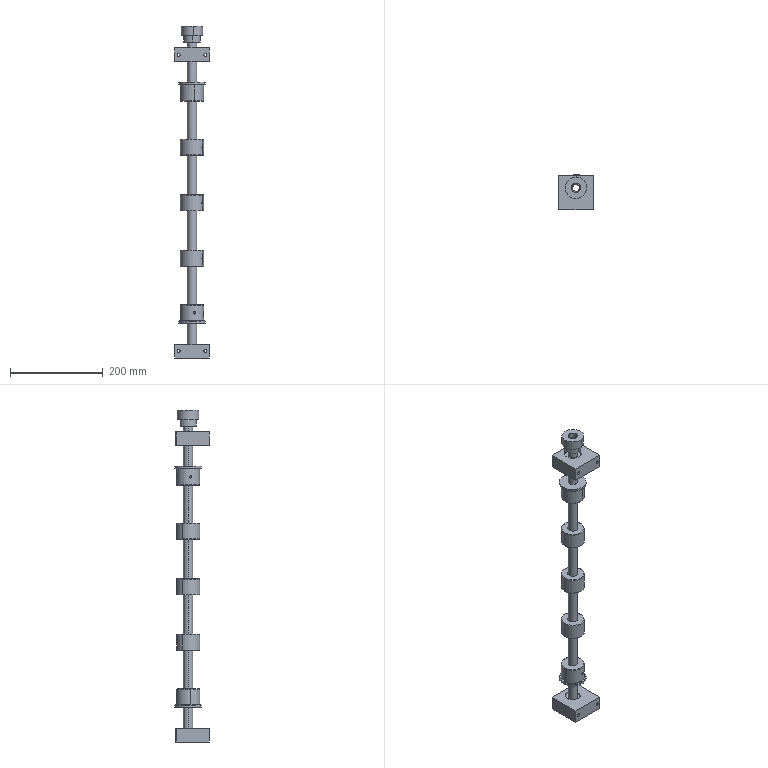Part | SolidWorks | 13 solids | 223 faces | box 74 x 75 x 717 mm | volume 685798 mm3 | cylinder 116 | plane 59 | cone 32 | torus 16 | commonest cylinder face diameters 20 x22 4.2 x20 5 x12 50 x10 6.6 x8 11 x8